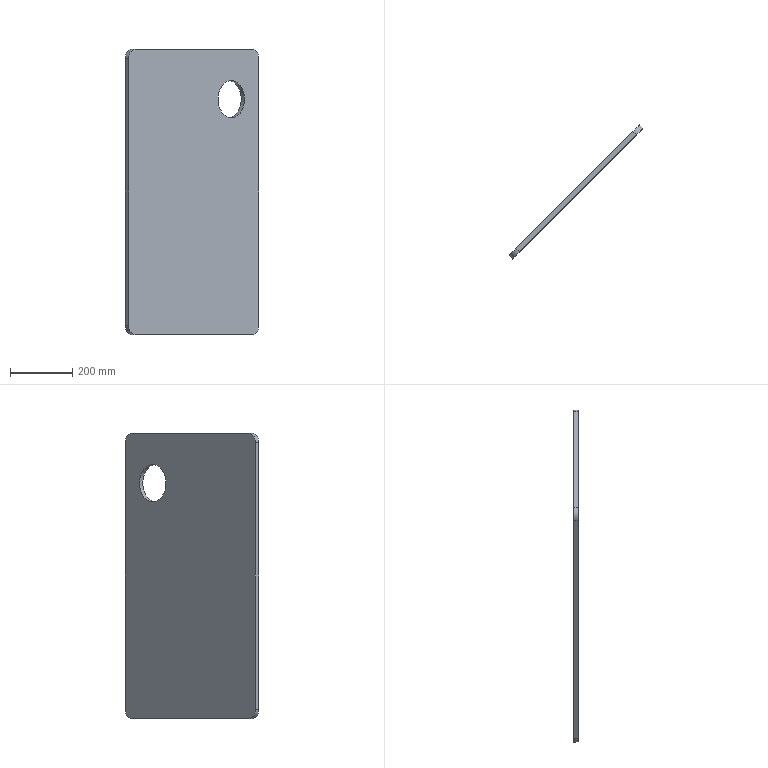Part | SolidWorks | 1 solid | 12 faces | box 429.306 x 429.306 x 917.42 mm | volume 7967244 mm3 | plane 6 | cylinder 6 | commonest cylinder face diameters 60 x4 120 x2
STEP:
#1=CARTESIAN_POINT('',(197.991,-424.263,65.));
#2=VERTEX_POINT('',#1);
#3=CARTESIAN_POINT('',(574.264,-47.99,65.));
#4=VERTEX_POINT('',#3);
#5=CARTESIAN_POINT('',(418.701,-203.553,65.));
#6=DIRECTION('',(0.7071,0.7071,0.));
#7=VECTOR('',#6,1000.);
#8=LINE('',#5,#7);
#9=EDGE_CURVE('',#2,#4,#8,.T.);
#10=ORIENTED_EDGE('',*,*,#9,.F.);
#11=CARTESIAN_POINT('',(208.598,-434.869,65.));
#12=VERTEX_POINT('',#11);
#13=CARTESIAN_POINT('',(-113.136,-113.136,65.));
#14=DIRECTION('',(0.7071,-0.7071,0.));
#15=VECTOR('',#14,1000.);
#16=LINE('',#13,#15);
#17=EDGE_CURVE('',#2,#12,#16,.T.);
#18=ORIENTED_EDGE('',*,*,#17,.T.);
#19=CARTESIAN_POINT('',(584.871,-58.597,65.));
#20=VERTEX_POINT('',#19);
#21=CARTESIAN_POINT('',(606.084,-37.383,65.));
#22=DIRECTION('',(-0.7071,-0.7071,0.));
#23=VECTOR('',#22,1000.);
#24=LINE('',#21,#23);
#25=EDGE_CURVE('',#20,#12,#24,.T.);
#26=ORIENTED_EDGE('',*,*,#25,.F.);
#27=CARTESIAN_POINT('',(263.137,263.137,65.));
#28=DIRECTION('',(-0.7071,0.7071,0.));
#29=VECTOR('',#28,1000.);
#30=LINE('',#27,#29);
#31=EDGE_CURVE('',#20,#4,#30,.T.);
#32=ORIENTED_EDGE('',*,*,#31,.T.);
#33=EDGE_LOOP('',(#10,#18,#26,#32));
#34=FACE_OUTER_BOUND('',#33,.T.);
#35=CARTESIAN_POINT('',(0.,0.,65.));
#36=DIRECTION('',(0.,0.,1.));
#37=DIRECTION('',(1.,0.,0.));
#38=AXIS2_PLACEMENT_3D('',#35,#36,#37);
#39=PLANE('',#38);
#40=ADVANCED_FACE('',(#34),#39,.T.);
#41=CARTESIAN_POINT('',(574.264,-47.99,-852.42));
#42=VERTEX_POINT('',#41);
#43=CARTESIAN_POINT('',(197.991,-424.263,-852.42));
#44=VERTEX_POINT('',#43);
#45=CARTESIAN_POINT('',(595.477,-26.777,-852.42));
#46=DIRECTION('',(-0.7071,-0.7071,0.));
#47=VECTOR('',#46,1000.);
#48=LINE('',#45,#47);
#49=EDGE_CURVE('',#42,#44,#48,.T.);
#50=ORIENTED_EDGE('',*,*,#49,.F.);
#51=CARTESIAN_POINT('',(584.871,-58.597,-852.42));
#52=VERTEX_POINT('',#51);
#53=CARTESIAN_POINT('',(263.137,263.137,-852.42));
#54=DIRECTION('',(0.7071,-0.7071,0.));
#55=VECTOR('',#54,1000.);
#56=LINE('',#53,#55);
#57=EDGE_CURVE('',#42,#52,#56,.T.);
#58=ORIENTED_EDGE('',*,*,#57,.T.);
#59=CARTESIAN_POINT('',(208.598,-434.869,-852.42));
#60=VERTEX_POINT('',#59);
#61=CARTESIAN_POINT('',(429.307,-214.16,-852.42));
#62=DIRECTION('',(0.7071,0.7071,0.));
#63=VECTOR('',#62,1000.);
#64=LINE('',#61,#63);
#65=EDGE_CURVE('',#60,#52,#64,.T.);
#66=ORIENTED_EDGE('',*,*,#65,.F.);
#67=CARTESIAN_POINT('',(-113.136,-113.136,-852.42));
#68=DIRECTION('',(-0.7071,0.7071,0.));
#69=VECTOR('',#68,1000.);
#70=LINE('',#67,#69);
#71=EDGE_CURVE('',#60,#44,#70,.T.);
#72=ORIENTED_EDGE('',*,*,#71,.T.);
#73=EDGE_LOOP('',(#50,#58,#66,#72));
#74=FACE_OUTER_BOUND('',#73,.T.);
#75=CARTESIAN_POINT('',(0.,0.,-852.42));
#76=DIRECTION('',(0.,0.,-1.));
#77=DIRECTION('',(0.,-1.,0.));
#78=AXIS2_PLACEMENT_3D('',#75,#76,#77);
#79=PLANE('',#78);
#80=ADVANCED_FACE('',(#74),#79,.T.);
#81=CARTESIAN_POINT('',(507.089,-115.165,-35.61));
#82=VERTEX_POINT('',#81);
#83=CARTESIAN_POINT('',(507.089,-115.165,-155.61));
#84=VERTEX_POINT('',#83);
#85=CARTESIAN_POINT('',(507.089,-115.165,-95.61));
#86=DIRECTION('',(-0.7071,0.7071,0.));
#87=DIRECTION('',(0.,0.,1.));
#88=AXIS2_PLACEMENT_3D('',#85,#86,#87);
#89=CIRCLE('',#88,60.);
#90=EDGE_CURVE('',#82,#84,#89,.T.);
#91=ORIENTED_EDGE('',*,*,#90,.F.);
#92=CARTESIAN_POINT('',(507.089,-115.165,-95.61));
#93=DIRECTION('',(-0.7071,0.7071,0.));
#94=DIRECTION('',(0.,0.,-1.));
#95=AXIS2_PLACEMENT_3D('',#92,#93,#94);
#96=CIRCLE('',#95,60.);
#97=EDGE_CURVE('',#84,#82,#96,.T.);
#98=ORIENTED_EDGE('',*,*,#97,.F.);
#99=EDGE_LOOP('',(#91,#98));
#100=FACE_BOUND('',#99,.T.);
#101=CARTESIAN_POINT('',(176.778,-445.476,35.));
#102=VERTEX_POINT('',#101);
#103=CARTESIAN_POINT('',(176.778,-445.476,-822.42));
#104=VERTEX_POINT('',#103);
#105=CARTESIAN_POINT('',(176.778,-445.476,65.));
#106=DIRECTION('',(0.,0.,-1.));
#107=VECTOR('',#106,1000.);
#108=LINE('',#105,#107);
#109=EDGE_CURVE('',#102,#104,#108,.T.);
#110=ORIENTED_EDGE('',*,*,#109,.F.);
#111=CARTESIAN_POINT('',(197.991,-424.263,35.));
#112=DIRECTION('',(-0.7071,0.7071,0.));
#113=DIRECTION('',(-0.7071,-0.7071,0.));
#114=AXIS2_PLACEMENT_3D('',#111,#112,#113);
#115=CIRCLE('',#114,30.);
#116=EDGE_CURVE('',#102,#2,#115,.T.);
#117=ORIENTED_EDGE('',*,*,#116,.T.);
#118=ORIENTED_EDGE('',*,*,#9,.T.);
#119=CARTESIAN_POINT('',(595.477,-26.777,35.));
#120=VERTEX_POINT('',#119);
#121=CARTESIAN_POINT('',(574.264,-47.99,35.));
#122=DIRECTION('',(-0.7071,0.7071,0.));
#123=DIRECTION('',(-0.7071,-0.7071,0.));
#124=AXIS2_PLACEMENT_3D('',#121,#122,#123);
#125=CIRCLE('',#124,30.);
#126=EDGE_CURVE('',#4,#120,#125,.T.);
#127=ORIENTED_EDGE('',*,*,#126,.T.);
#128=CARTESIAN_POINT('',(595.477,-26.777,-822.42));
#129=VERTEX_POINT('',#128);
#130=CARTESIAN_POINT('',(595.477,-26.777,65.));
#131=DIRECTION('',(0.,0.,-1.));
#132=VECTOR('',#131,1000.);
#133=LINE('',#130,#132);
#134=EDGE_CURVE('',#120,#129,#133,.T.);
#135=ORIENTED_EDGE('',*,*,#134,.T.);
#136=CARTESIAN_POINT('',(574.264,-47.99,-822.42));
#137=DIRECTION('',(-0.7071,0.7071,0.));
#138=DIRECTION('',(-0.7071,-0.7071,0.));
#139=AXIS2_PLACEMENT_3D('',#136,#137,#138);
#140=CIRCLE('',#139,30.);
#141=EDGE_CURVE('',#129,#42,#140,.T.);
#142=ORIENTED_EDGE('',*,*,#141,.T.);
#143=ORIENTED_EDGE('',*,*,#49,.T.);
#144=CARTESIAN_POINT('',(197.991,-424.263,-822.42));
#145=DIRECTION('',(-0.7071,0.7071,0.));
#146=DIRECTION('',(-0.7071,-0.7071,0.));
#147=AXIS2_PLACEMENT_3D('',#144,#145,#146);
#148=CIRCLE('',#147,30.);
#149=EDGE_CURVE('',#44,#104,#148,.T.);
#150=ORIENTED_EDGE('',*,*,#149,.T.);
#151=EDGE_LOOP('',(#110,#117,#118,#127,#135,#142,#143,#150));
#152=FACE_OUTER_BOUND('',#151,.T.);
#153=CARTESIAN_POINT('',(418.701,-203.553,-852.42));
#154=DIRECTION('',(-0.7071,0.7071,0.));
#155=DIRECTION('',(0.,0.,1.));
#156=AXIS2_PLACEMENT_3D('',#153,#154,#155);
#157=PLANE('',#156);
#158=ADVANCED_FACE('',(#100,#152),#157,.T.);
#159=CARTESIAN_POINT('',(606.084,-37.383,35.));
#160=VERTEX_POINT('',#159);
#161=CARTESIAN_POINT('',(606.084,-37.383,-822.42));
#162=VERTEX_POINT('',#161);
#163=CARTESIAN_POINT('',(606.084,-37.383,65.));
#164=DIRECTION('',(0.,0.,-1.));
#165=VECTOR('',#164,1000.);
#166=LINE('',#163,#165);
#167=EDGE_CURVE('',#160,#162,#166,.T.);
#168=ORIENTED_EDGE('',*,*,#167,.T.);
#169=CARTESIAN_POINT('',(595.477,-26.777,-822.42));
#170=DIRECTION('',(-0.7071,0.7071,0.));
#171=VECTOR('',#170,1000.);
#172=LINE('',#169,#171);
#173=EDGE_CURVE('',#162,#129,#172,.T.);
#174=ORIENTED_EDGE('',*,*,#173,.T.);
#175=ORIENTED_EDGE('',*,*,#134,.F.);
#176=CARTESIAN_POINT('',(595.477,-26.777,35.));
#177=DIRECTION('',(0.7071,-0.7071,0.));
#178=VECTOR('',#177,1000.);
#179=LINE('',#176,#178);
#180=EDGE_CURVE('',#120,#160,#179,.T.);
#181=ORIENTED_EDGE('',*,*,#180,.T.);
#182=EDGE_LOOP('',(#168,#174,#175,#181));
#183=FACE_OUTER_BOUND('',#182,.T.);
#184=CARTESIAN_POINT('',(595.477,-26.777,-852.42));
#185=DIRECTION('',(0.7071,0.7071,0.));
#186=DIRECTION('',(0.,0.,-1.));
#187=AXIS2_PLACEMENT_3D('',#184,#185,#186);
#188=PLANE('',#187);
#189=ADVANCED_FACE('',(#183),#188,.T.);
#190=CARTESIAN_POINT('',(517.696,-125.772,-155.61));
#191=VERTEX_POINT('',#190);
#192=CARTESIAN_POINT('',(517.696,-125.772,-35.61));
#193=VERTEX_POINT('',#192);
#194=CARTESIAN_POINT('',(517.696,-125.772,-95.61));
#195=DIRECTION('',(0.7071,-0.7071,0.));
#196=DIRECTION('',(0.,0.,-1.));
#197=AXIS2_PLACEMENT_3D('',#194,#195,#196);
#198=CIRCLE('',#197,60.);
#199=EDGE_CURVE('',#191,#193,#198,.T.);
#200=ORIENTED_EDGE('',*,*,#199,.F.);
#201=CARTESIAN_POINT('',(517.696,-125.772,-95.61));
#202=DIRECTION('',(0.7071,-0.7071,0.));
#203=DIRECTION('',(0.,0.,1.));
#204=AXIS2_PLACEMENT_3D('',#201,#202,#203);
#205=CIRCLE('',#204,60.);
#206=EDGE_CURVE('',#193,#191,#205,.T.);
#207=ORIENTED_EDGE('',*,*,#206,.F.);
#208=EDGE_LOOP('',(#200,#207));
#209=FACE_BOUND('',#208,.T.);
#210=ORIENTED_EDGE('',*,*,#25,.T.);
#211=CARTESIAN_POINT('',(187.385,-456.082,35.));
#212=VERTEX_POINT('',#211);
#213=CARTESIAN_POINT('',(208.598,-434.869,35.));
#214=DIRECTION('',(0.7071,-0.7071,0.));
#215=DIRECTION('',(0.7071,0.7071,0.));
#216=AXIS2_PLACEMENT_3D('',#213,#214,#215);
#217=CIRCLE('',#216,30.);
#218=EDGE_CURVE('',#12,#212,#217,.T.);
#219=ORIENTED_EDGE('',*,*,#218,.T.);
#220=CARTESIAN_POINT('',(187.385,-456.082,-822.42));
#221=VERTEX_POINT('',#220);
#222=CARTESIAN_POINT('',(187.385,-456.082,-852.42));
#223=DIRECTION('',(0.,0.,1.));
#224=VECTOR('',#223,1000.);
#225=LINE('',#222,#224);
#226=EDGE_CURVE('',#221,#212,#225,.T.);
#227=ORIENTED_EDGE('',*,*,#226,.F.);
#228=CARTESIAN_POINT('',(208.598,-434.869,-822.42));
#229=DIRECTION('',(0.7071,-0.7071,0.));
#230=DIRECTION('',(0.7071,0.7071,0.));
#231=AXIS2_PLACEMENT_3D('',#228,#229,#230);
#232=CIRCLE('',#231,30.);
#233=EDGE_CURVE('',#221,#60,#232,.T.);
#234=ORIENTED_EDGE('',*,*,#233,.T.);
#235=ORIENTED_EDGE('',*,*,#65,.T.);
#236=CARTESIAN_POINT('',(584.871,-58.597,-822.42));
#237=DIRECTION('',(0.7071,-0.7071,0.));
#238=DIRECTION('',(0.7071,0.7071,0.));
#239=AXIS2_PLACEMENT_3D('',#236,#237,#238);
#240=CIRCLE('',#239,30.);
#241=EDGE_CURVE('',#52,#162,#240,.T.);
#242=ORIENTED_EDGE('',*,*,#241,.T.);
#243=ORIENTED_EDGE('',*,*,#167,.F.);
#244=CARTESIAN_POINT('',(584.871,-58.597,35.));
#245=DIRECTION('',(0.7071,-0.7071,0.));
#246=DIRECTION('',(0.7071,0.7071,0.));
#247=AXIS2_PLACEMENT_3D('',#244,#245,#246);
#248=CIRCLE('',#247,30.);
#249=EDGE_CURVE('',#160,#20,#248,.T.);
#250=ORIENTED_EDGE('',*,*,#249,.T.);
#251=EDGE_LOOP('',(#210,#219,#227,#234,#235,#242,#243,#250));
#252=FACE_OUTER_BOUND('',#251,.T.);
#253=CARTESIAN_POINT('',(606.084,-37.383,-852.42));
#254=DIRECTION('',(0.7071,-0.7071,0.));
#255=DIRECTION('',(0.,0.,-1.));
#256=AXIS2_PLACEMENT_3D('',#253,#254,#255);
#257=PLANE('',#256);
#258=ADVANCED_FACE('',(#209,#252),#257,.T.);
#259=ORIENTED_EDGE('',*,*,#90,.T.);
#260=CARTESIAN_POINT('',(507.089,-115.165,-155.61));
#261=DIRECTION('',(0.7071,-0.7071,0.));
#262=VECTOR('',#261,1000.);
#263=LINE('',#260,#262);
#264=EDGE_CURVE('',#84,#191,#263,.T.);
#265=ORIENTED_EDGE('',*,*,#264,.T.);
#266=ORIENTED_EDGE('',*,*,#199,.T.);
#267=CARTESIAN_POINT('',(507.089,-115.165,-35.61));
#268=DIRECTION('',(0.7071,-0.7071,0.));
#269=VECTOR('',#268,1000.);
#270=LINE('',#267,#269);
#271=EDGE_CURVE('',#82,#193,#270,.T.);
#272=ORIENTED_EDGE('',*,*,#271,.F.);
#273=EDGE_LOOP('',(#259,#265,#266,#272));
#274=FACE_OUTER_BOUND('',#273,.T.);
#275=CARTESIAN_POINT('',(517.696,-125.772,-95.61));
#276=DIRECTION('',(0.7071,-0.7071,0.));
#277=DIRECTION('',(0.,0.,-1.));
#278=AXIS2_PLACEMENT_3D('',#275,#276,#277);
#279=CYLINDRICAL_SURFACE('',#278,60.);
#280=ADVANCED_FACE('',(#274),#279,.F.);
#281=ORIENTED_EDGE('',*,*,#97,.T.);
#282=ORIENTED_EDGE('',*,*,#271,.T.);
#283=ORIENTED_EDGE('',*,*,#206,.T.);
#284=ORIENTED_EDGE('',*,*,#264,.F.);
#285=EDGE_LOOP('',(#281,#282,#283,#284));
#286=FACE_OUTER_BOUND('',#285,.T.);
#287=CARTESIAN_POINT('',(517.696,-125.772,-95.61));
#288=DIRECTION('',(0.7071,-0.7071,0.));
#289=DIRECTION('',(0.,0.,-1.));
#290=AXIS2_PLACEMENT_3D('',#287,#288,#289);
#291=CYLINDRICAL_SURFACE('',#290,60.);
#292=ADVANCED_FACE('',(#286),#291,.F.);
#293=ORIENTED_EDGE('',*,*,#226,.T.);
#294=CARTESIAN_POINT('',(-134.349,-134.349,35.));
#295=DIRECTION('',(-0.7071,0.7071,0.));
#296=VECTOR('',#295,1000.);
#297=LINE('',#294,#296);
#298=EDGE_CURVE('',#212,#102,#297,.T.);
#299=ORIENTED_EDGE('',*,*,#298,.T.);
#300=ORIENTED_EDGE('',*,*,#109,.T.);
#301=CARTESIAN_POINT('',(-134.349,-134.349,-822.42));
#302=DIRECTION('',(0.7071,-0.7071,0.));
#303=VECTOR('',#302,1000.);
#304=LINE('',#301,#303);
#305=EDGE_CURVE('',#104,#221,#304,.T.);
#306=ORIENTED_EDGE('',*,*,#305,.T.);
#307=EDGE_LOOP('',(#293,#299,#300,#306));
#308=FACE_OUTER_BOUND('',#307,.T.);
#309=CARTESIAN_POINT('',(-134.349,-134.349,0.));
#310=DIRECTION('',(-0.7071,-0.7071,0.));
#311=DIRECTION('',(0.7071,-0.7071,0.));
#312=AXIS2_PLACEMENT_3D('',#309,#310,#311);
#313=PLANE('',#312);
#314=ADVANCED_FACE('',(#308),#313,.T.);
#315=ORIENTED_EDGE('',*,*,#218,.F.);
#316=ORIENTED_EDGE('',*,*,#17,.F.);
#317=ORIENTED_EDGE('',*,*,#116,.F.);
#318=ORIENTED_EDGE('',*,*,#298,.F.);
#319=EDGE_LOOP('',(#315,#316,#317,#318));
#320=FACE_OUTER_BOUND('',#319,.T.);
#321=CARTESIAN_POINT('',(-113.136,-113.136,35.));
#322=DIRECTION('',(-0.7071,0.7071,0.));
#323=DIRECTION('',(-0.7071,-0.7071,0.));
#324=AXIS2_PLACEMENT_3D('',#321,#322,#323);
#325=CYLINDRICAL_SURFACE('',#324,30.);
#326=ADVANCED_FACE('',(#320),#325,.T.);
#327=ORIENTED_EDGE('',*,*,#241,.F.);
#328=ORIENTED_EDGE('',*,*,#57,.F.);
#329=ORIENTED_EDGE('',*,*,#141,.F.);
#330=ORIENTED_EDGE('',*,*,#173,.F.);
#331=EDGE_LOOP('',(#327,#328,#329,#330));
#332=FACE_OUTER_BOUND('',#331,.T.);
#333=CARTESIAN_POINT('',(574.264,-47.99,-822.42));
#334=DIRECTION('',(-0.7071,0.7071,0.));
#335=DIRECTION('',(-0.7071,-0.7071,0.));
#336=AXIS2_PLACEMENT_3D('',#333,#334,#335);
#337=CYLINDRICAL_SURFACE('',#336,30.);
#338=ADVANCED_FACE('',(#332),#337,.T.);
#339=ORIENTED_EDGE('',*,*,#126,.F.);
#340=ORIENTED_EDGE('',*,*,#31,.F.);
#341=ORIENTED_EDGE('',*,*,#249,.F.);
#342=ORIENTED_EDGE('',*,*,#180,.F.);
#343=EDGE_LOOP('',(#339,#340,#341,#342));
#344=FACE_OUTER_BOUND('',#343,.T.);
#345=CARTESIAN_POINT('',(574.264,-47.99,35.));
#346=DIRECTION('',(0.7071,-0.7071,0.));
#347=DIRECTION('',(0.7071,0.7071,0.));
#348=AXIS2_PLACEMENT_3D('',#345,#346,#347);
#349=CYLINDRICAL_SURFACE('',#348,30.);
#350=ADVANCED_FACE('',(#344),#349,.T.);
#351=ORIENTED_EDGE('',*,*,#149,.F.);
#352=ORIENTED_EDGE('',*,*,#71,.F.);
#353=ORIENTED_EDGE('',*,*,#233,.F.);
#354=ORIENTED_EDGE('',*,*,#305,.F.);
#355=EDGE_LOOP('',(#351,#352,#353,#354));
#356=FACE_OUTER_BOUND('',#355,.T.);
#357=CARTESIAN_POINT('',(-113.136,-113.136,-822.42));
#358=DIRECTION('',(0.7071,-0.7071,0.));
#359=DIRECTION('',(0.7071,0.7071,0.));
#360=AXIS2_PLACEMENT_3D('',#357,#358,#359);
#361=CYLINDRICAL_SURFACE('',#360,30.);
#362=ADVANCED_FACE('',(#356),#361,.T.);
#363=CLOSED_SHELL('',(#40,#80,#158,#189,#258,#280,#292,#314,#326,#338,#350,#362));
#364=MANIFOLD_SOLID_BREP('',#363);
#365=CARTESIAN_POINT('',(0.,0.,0.));
#366=DIRECTION('',(0.,0.,1.));
#367=DIRECTION('',(1.,0.,0.));
#368=AXIS2_PLACEMENT_3D('',#365,#366,#367);
#369=(LENGTH_UNIT()NAMED_UNIT(*)SI_UNIT(.MILLI.,.METRE.));
#370=UNCERTAINTY_MEASURE_WITH_UNIT(LENGTH_MEASURE(0.00001),#369,'','');
#371=(NAMED_UNIT(*)PLANE_ANGLE_UNIT()SI_UNIT($,.RADIAN.));
#372=(NAMED_UNIT(*)SI_UNIT($,.STERADIAN.)SOLID_ANGLE_UNIT());
#373=(GEOMETRIC_REPRESENTATION_CONTEXT(3)GLOBAL_UNCERTAINTY_ASSIGNED_CONTEXT((#370))GLOBAL_UNIT_ASSIGNED_CONTEXT((#369,#371,#372))REPRESENTATION_CONTEXT('',''));
#374=ADVANCED_BREP_SHAPE_REPRESENTATION('',(#364,#368),#373);